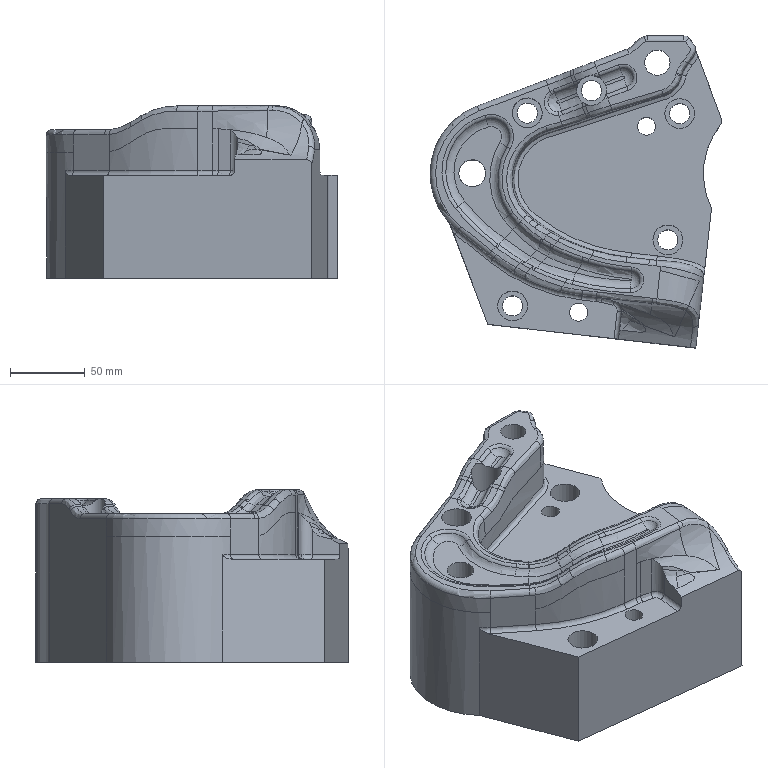Part | NX | features 23 2 | 1 solid | 218 faces | box 195.229 x 209 x 115.4 mm | volume 2400595 mm3 | spline 86 | cylinder 61 | plane 37 | torus 34 | commonest cylinder face diameters 7 x10 6 x8 13.5 x5 20 x5 13 x4 10 x2